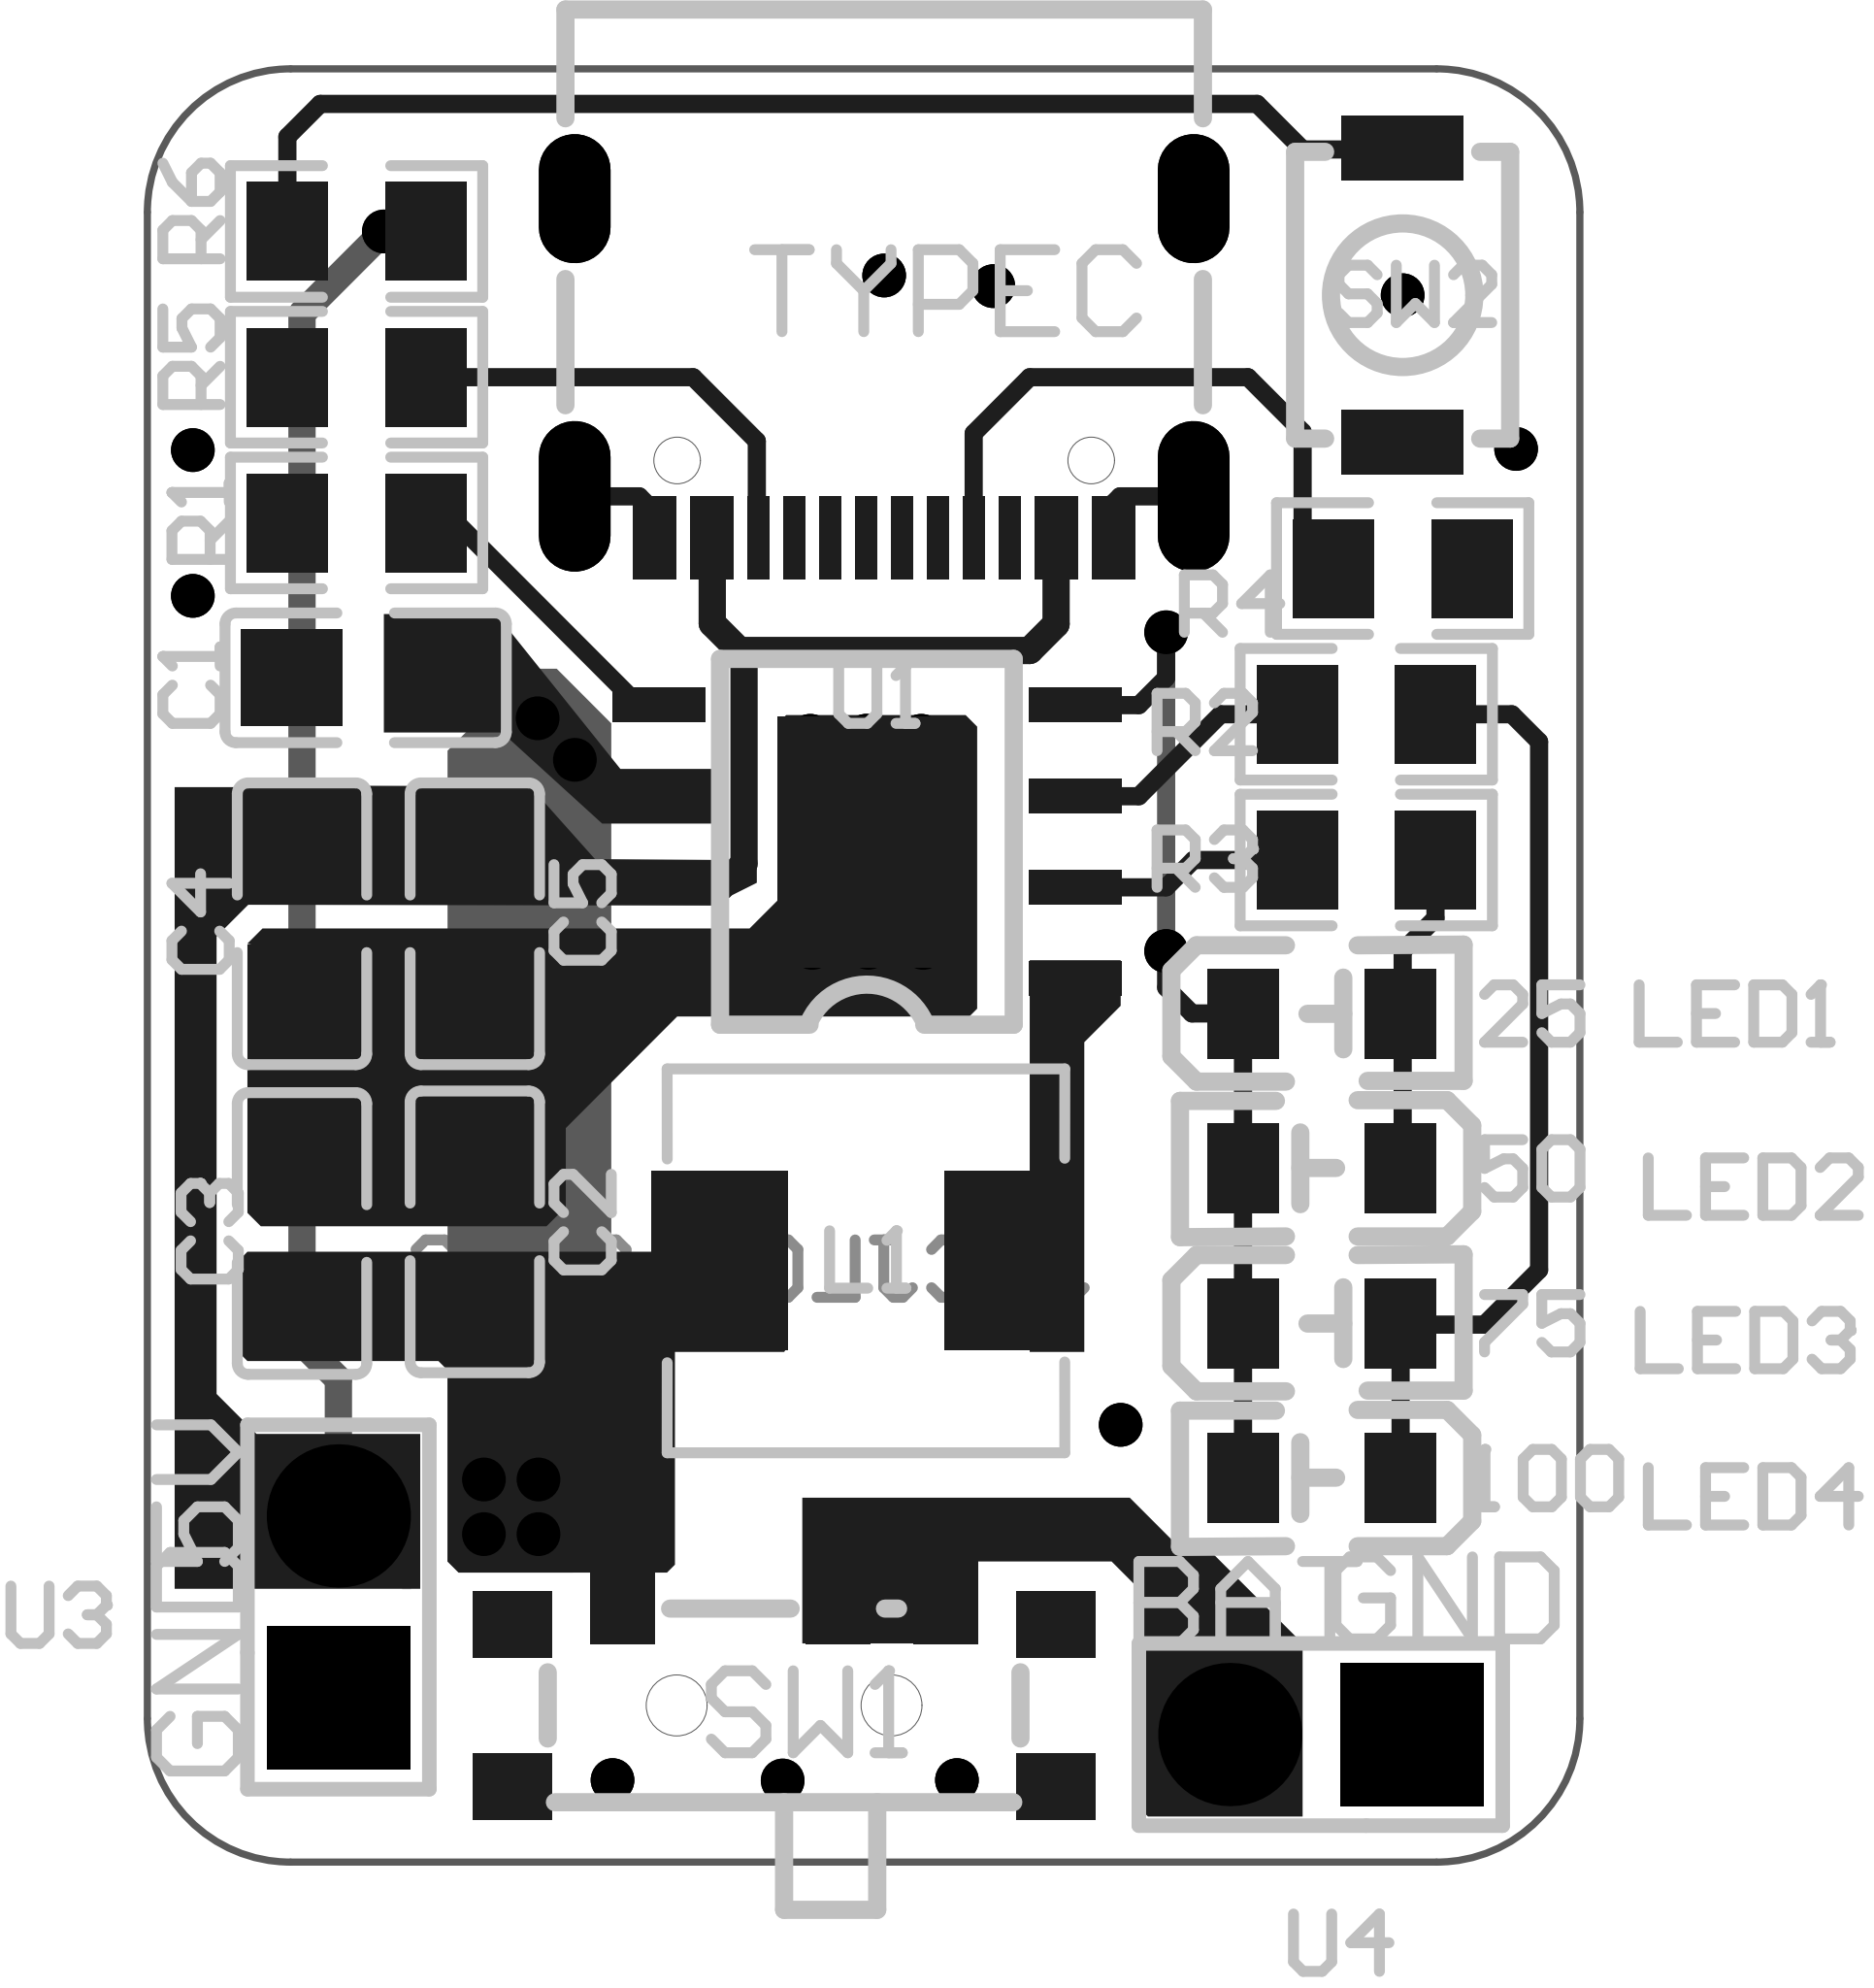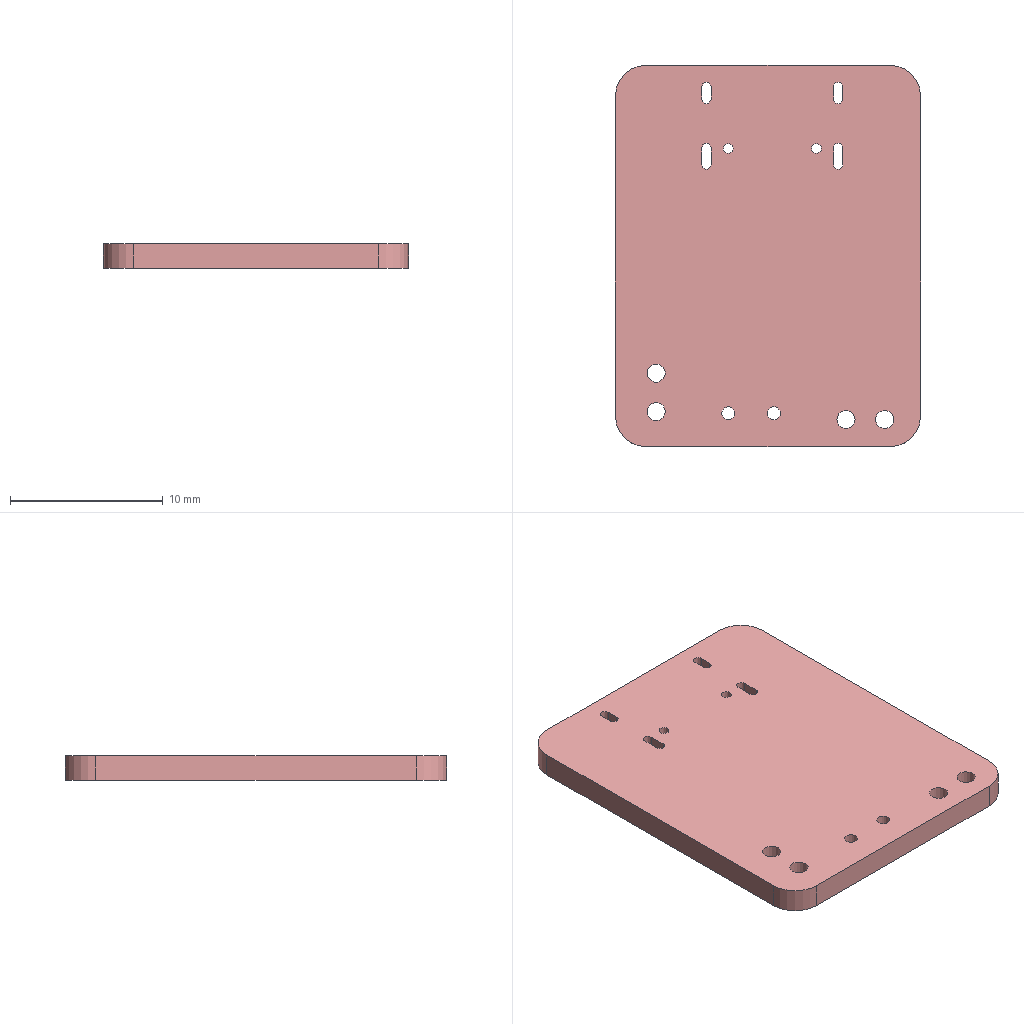Circuit board layout | Altium Designer | box 20 x 25 x 1.6 mm
Layer stack:
# Altium Designer layer stack of  (unit mm; dielectric type: 0 none, 1 core, 2 prepreg, 3 surface material)
index,name,kind,layer,copper_thickness_mm,dielectric_type,dielectric_thickness_mm,dielectric_material,dielectric_constant
0,Top Paste Mask Layer,other,,,,,,
1,Top Silkscreen Layer,other,,,,,,
2,Top Solder Mask Layer,dielectric,,,3,0.01,,3.3
3,Top Layer,copper,Top Layer,0.035,,,,
4,Dielectric1,dielectric,,,3,1.51,FR4,4.5
5,Bottom Layer,copper,Bottom Layer,0.035,,,,
6,Bottom Solder Mask Layer,dielectric,,,3,0.01,,3.3
7,Bottom Silkscreen Layer,other,,,,,,
8,Bottom Paste Mask Layer,other,,,,,,
# drill layer pairs: low layer,high layer
drill_pair,Top Layer,Bottom Layer
Part placement:
Designator,Comment,Layer,Footprint,Center-X(mm),Center-Y(mm),Rotation
L1,2.2uH,TopLayer,IND-SMD_L5.4-W5.2,90.043,87.757,0
R4,5.1KΩ,TopLayer,R0805,97.536,97.409,180
R5,5.1KΩ,TopLayer,R0805,82.931,100.076,0
R6,51Ω,TopLayer,R0805,82.931,102.108,180
C1,1uF,TopLayer,C0805,83.058,95.885,180
C2,22uF,TopLayer,C0805,84.582,88.161,270
R1,75KΩ,TopLayer,R0805,82.931,98.044,0
C3,22uF,TopLayer,C0805,82.169,88.138,270
C4,22uF,TopLayer,C0805,82.169,92.456,90
C5,22uF,TopLayer,C0805,84.582,92.456,90
LED4,led0805,TopLayer,LED0805-RD,96.407,84.729,180
LED3,led0805,TopLayer,LED0805-RD,96.407,86.888,0
R2,1kΩ,TopLayer,R0805,97.028,95.377,180
R3,1kΩ,TopLayer,R0805,97.028,93.345,180
LED2,led0805,TopLayer,LED0805-RD,96.407,89.047,180
LED1,led0805,TopLayer,LED0805-RD,96.407,91.206,0
SW1,MK-12C02-G015,TopLayer,SW-SMD_G-SWITCH_MK-12C02-G015,88.9,81.915,0
TYPEC,TYPE-C 16PIN 3MD(385),TopLayer,USB-C-SMD_TYPE-C16PIN,90.297,100.203,180
SW2,ST-1185U,TopLayer,SW-SMD_ST-1185U,97.536,101.219,270
U3,2.54-1*2,TopLayer,HDR-TH_2P-P2.54-V-M,82.677,82.931,90
U4,2.54-1*2,TopLayer,HDR-TH_2P-P2.54-V-M,96.393,81.153,180
U1,ETA9740,TopLayer,ESOP-8,90.056,93.599,180
Pad and via stacks:
# Altium Designer via and pad stacks of  (unit mm). Each distinct definition once, with the count of objects using it.
# via: kind,start_layer,end_layer,hole_mm,diameter_mm,mode(0 simple;1 top-mid-bottom;2 full stack),diameter_per_layer,count,example_net
# pad: kind,layer,hole_mm,hole_type(0 round;1 square;2 slot),plating,top_size,top_shape(1 round;2 rect;3 octagon;9 rounded rect),mid_size,bottom_size,mode,footprint,size_per_layer,count,example
pad,Top Layer,0,0,plated,1.9x2.5,2,1.9x2.5,1.9x2.5,0,IND-SMD_L5.4-W5.2,,2,L1.1
pad,Top Layer,0,0,plated,1.133x1.377,2,1.133x1.377,1.133x1.377,0,R0805,,12,R4.2
pad,Top Layer,0,0,plated,1.41x1.35,2,1.41x1.35,1.41x1.35,0,C0805,,10,C1.2
pad,Top Layer,0,0,plated,1x1.25,2,1x1.25,1x1.25,0,LED0805-RD,,8,LED4.2
pad,Top Layer,0,0,plated,0.9x2,2,0.9x2,0.9x2,0,SW-SMD_G-SWITCH_MK-12C02-G015,,3,SW1.1
pad,Top Layer,0,0,plated,1.1x0.93,2,1.1x0.93,1.1x0.93,0,SW-SMD_G-SWITCH_MK-12C02-G015,,4,SW1.4
pad,Top Layer,0,0,plated,0.5994x1.151,2,0.5994x1.151,0.5994x1.151,0,USB-C-SMD_TYPE-C16PIN,,4,TYPEC.A1B12
pad,Top Layer,0,0,plated,0.2997x1.151,2,0.2997x1.151,0.2997x1.151,0,USB-C-SMD_TYPE-C16PIN,,8,TYPEC.B5
pad,Top Layer,0,0,plated,0.8992x1.699,2,0.8992x1.699,0.8992x1.699,0,SW-SMD_ST-1185U,,2,SW2.1
pad,Top Layer,0,0,plated,1.3x0.4801,2,1.3x0.4801,1.3x0.4801,0,ESOP-8,,8,U1.8
pad,Top Layer,0,0,plated,3.5x2.5,2,3.5x2.5,3.5x2.5,0,ESOP-8,,1,U1.9
pad,Multi-Layer,0.5994,2,plated,1.001x1.801,1,1.001x1.801,1.001x1.801,0,USB-C-SMD_TYPE-C16PIN,,2,TYPEC.4
pad,Multi-Layer,0.5994,2,plated,1.001x2.101,1,1.001x2.101,1.001x2.101,0,USB-C-SMD_TYPE-C16PIN,,2,TYPEC.2
pad,Multi-Layer,1.2,0,plated,2x2,2,2x2,2x2,0,HDR-TH_2P-P2.54-V-M,,2,U3.1
pad,Multi-Layer,1.2,0,plated,2x2,1,2x2,2x2,0,HDR-TH_2P-P2.54-V-M,,2,U3.2
via,Top Layer,Bottom Layer,0.3048,0.61,0,,34,$1N17516
Copper pours:
name,layer,net,type(0 solid;1 hatched;2 none)
Top Layer-GND,Top Layer,GND,0
Bottom Layer-GND,Bottom Layer,GND,0
Design rules, without the lines most boards share:
# Altium Designer design rules of  (exported by Altium Designer, unit mm)
# columns: name | kind | enabled | priority | scope1 | scope2 | descriptor | typed fields (field=value)
Plane_innerPlane | 0 | disabled | 1 | All | All | Clearance Constraint (Gap=6mil) (Disabled)(All),(All) | gap=0.1524
Plane_innerPlane_1 | 63 | disabled | 1 | All | All | Board Clearance Constraint (Gap=0mil) (Disabled)(All) |
Copper_copperRegion | 0 | disabled | 2 | All | All | Clearance Constraint (Gap=6mil) (Disabled)(All),(All) | gap=0.1524
Copper_copperRegion_1 | 63 | disabled | 2 | All | All | Board Clearance Constraint (Gap=0mil) (Disabled)(All) |
safeClearance | 0 | enabled | 3 | All | All | Clearance Constraint (Gap=6mil) (All),(All) | gap=0.1524
safeClearance_1 | 63 | enabled | 3 | All | All | Board Clearance Constraint (Gap=0mil) (All) |
otherClearance | 52 | enabled | 1 | All | All | Hole To Hole Clearance (Gap=11.8mil) (All),(All) | gap=0.2997
trackWidth | 2 | enabled | 1 | All | All | Width Constraint (Min=5mil) (Max=100mil) (Preferred=10mil) (All) |
viaSize | 11 | enabled | 1 | All | All | Routing Via (MinHoleWidth=11.811mil) (MaxHoleWidth=236.22mil) (PreferredHoleWidth=12.008mil) (MinWidth=19.685mil) (MaxWidth=393.701mil) (PreferedWidth=24.016mil) (All) | via_min_hole=0.3 via_max_hole=6 via_preferred_diameter=0.61 via_preferred_hole=0.305
solderMaskExpansion | 13 | enabled | 2 | All | All | Solder Mask Expansion (Expansion =4mil) (All) | expansion=0.1016